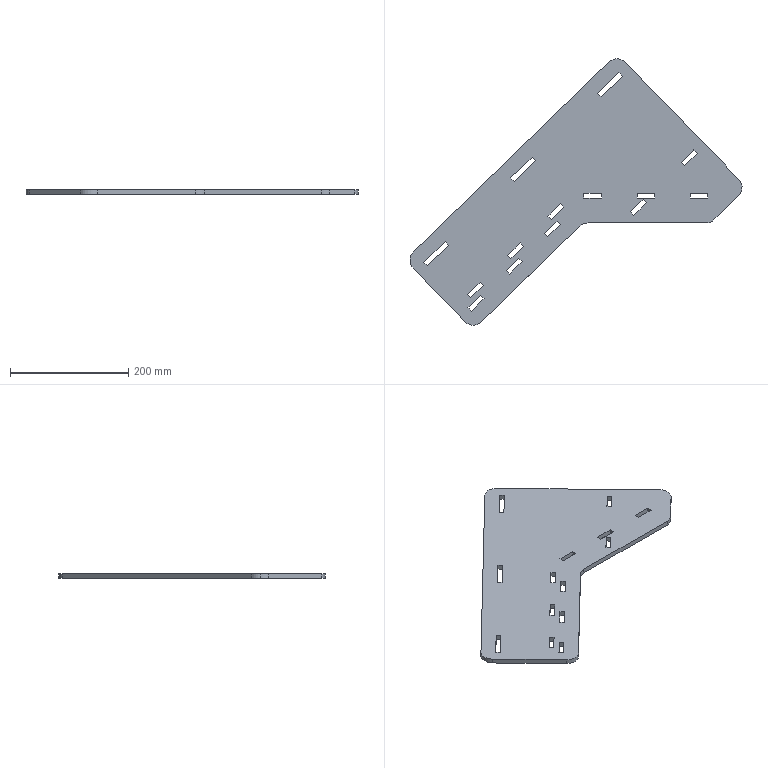Part | SolidWorks | features FlatPattern 1, SMBaseFlange 1, SheetMetal 1 | 1 solid | 71 faces | box 561.534 x 450.241 x 8 mm | volume 822286 mm3 | plane 64 | cylinder 7 | commonest cylinder face diameters 40 x7